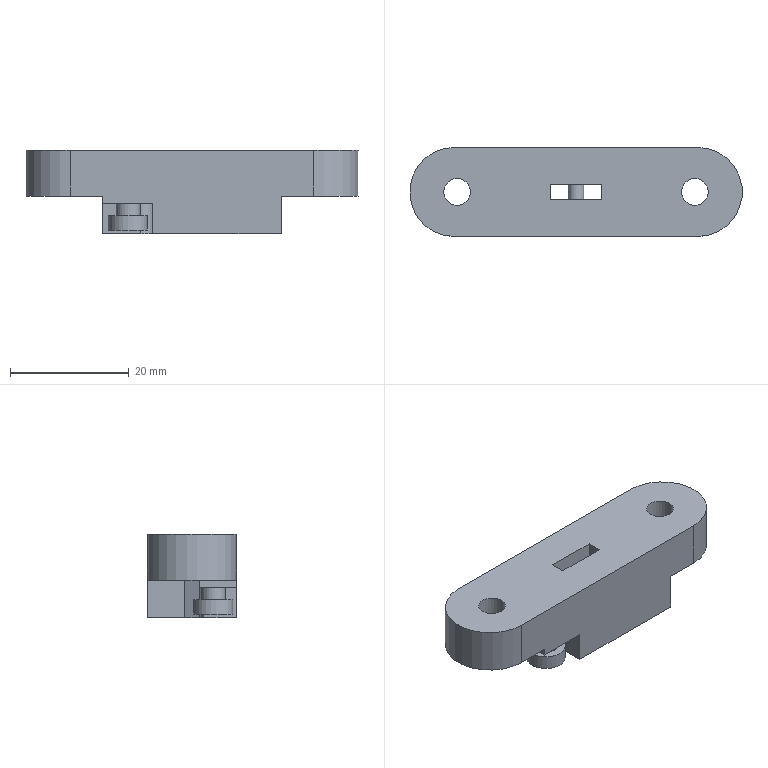Part | NX | 1 solid | 39 faces | box 56 x 15 x 14 mm | volume 7520 mm3 | plane 28 | cylinder 9 | cone 2 | commonest cylinder face diameters 2.7 x2 4 x2 4.5 x2 15 x2 6.6 x1
STEP:
#1=CARTESIAN_POINT('',(2.4,79.3,36.5));
#2=VERTEX_POINT('',#1);
#3=CARTESIAN_POINT('',(4.4,78.54,36.5));
#4=VERTEX_POINT('',#3);
#5=CARTESIAN_POINT('',(4.,80.5,36.5));
#6=DIRECTION('',(0.,0.,-1.));
#7=DIRECTION('',(0.,-1.,0.));
#8=AXIS2_PLACEMENT_3D('',#5,#6,#7);
#9=CIRCLE('',#8,2.);
#10=EDGE_CURVE('',#2,#4,#9,.F.);
#11=ORIENTED_EDGE('',*,*,#10,.T.);
#12=CARTESIAN_POINT('',(4.4,73.,36.5));
#13=VERTEX_POINT('',#12);
#14=CARTESIAN_POINT('',(4.4,79.3,36.5));
#15=DIRECTION('',(0.,-1.,0.));
#16=VECTOR('',#15,1000.);
#17=LINE('',#14,#16);
#18=EDGE_CURVE('',#4,#13,#17,.T.);
#19=ORIENTED_EDGE('',*,*,#18,.T.);
#20=CARTESIAN_POINT('',(-4.,73.,36.5));
#21=VERTEX_POINT('',#20);
#22=CARTESIAN_POINT('',(-4.,73.,36.5));
#23=DIRECTION('',(-1.,0.,0.));
#24=VECTOR('',#23,1000.);
#25=LINE('',#22,#24);
#26=EDGE_CURVE('',#13,#21,#25,.T.);
#27=ORIENTED_EDGE('',*,*,#26,.T.);
#28=CARTESIAN_POINT('',(-4.,79.3,36.5));
#29=VERTEX_POINT('',#28);
#30=CARTESIAN_POINT('',(-4.,79.3,36.5));
#31=DIRECTION('',(0.,1.,0.));
#32=VECTOR('',#31,1000.);
#33=LINE('',#30,#32);
#34=EDGE_CURVE('',#21,#29,#33,.T.);
#35=ORIENTED_EDGE('',*,*,#34,.T.);
#36=CARTESIAN_POINT('',(-4.,79.3,36.5));
#37=DIRECTION('',(1.,0.,0.));
#38=VECTOR('',#37,1000.);
#39=LINE('',#36,#38);
#40=EDGE_CURVE('',#29,#2,#39,.T.);
#41=ORIENTED_EDGE('',*,*,#40,.T.);
#42=EDGE_LOOP('',(#11,#19,#27,#35,#41));
#43=FACE_BOUND('',#42,.T.);
#44=CARTESIAN_POINT('',(0.2,74.9,36.5));
#45=VERTEX_POINT('',#44);
#46=CARTESIAN_POINT('',(0.2,76.9,36.5));
#47=DIRECTION('',(0.,0.,-1.));
#48=DIRECTION('',(0.,-1.,0.));
#49=AXIS2_PLACEMENT_3D('',#46,#47,#48);
#50=CIRCLE('',#49,2.);
#51=EDGE_CURVE('',#45,#45,#50,.T.);
#52=ORIENTED_EDGE('',*,*,#51,.F.);
#53=EDGE_LOOP('',(#52));
#54=FACE_BOUND('',#53,.T.);
#55=CARTESIAN_POINT('',(4.4,79.3,36.5));
#56=DIRECTION('',(0.,0.,-1.));
#57=DIRECTION('',(0.,-1.,0.));
#58=AXIS2_PLACEMENT_3D('',#55,#56,#57);
#59=PLANE('',#58);
#60=ADVANCED_FACE('',(#43,#54),#59,.T.);
#61=ORIENTED_EDGE('',*,*,#34,.F.);
#62=CARTESIAN_POINT('',(-4.,73.,37.7));
#63=VERTEX_POINT('',#62);
#64=CARTESIAN_POINT('',(-4.,73.,31.4));
#65=DIRECTION('',(0.,0.,1.));
#66=VECTOR('',#65,1000.);
#67=LINE('',#64,#66);
#68=EDGE_CURVE('',#21,#63,#67,.T.);
#69=ORIENTED_EDGE('',*,*,#68,.T.);
#70=CARTESIAN_POINT('',(-4.,79.3,37.7));
#71=VERTEX_POINT('',#70);
#72=CARTESIAN_POINT('',(-4.,88.,37.7));
#73=DIRECTION('',(0.,1.,0.));
#74=VECTOR('',#73,1000.);
#75=LINE('',#72,#74);
#76=EDGE_CURVE('',#63,#71,#75,.T.);
#77=ORIENTED_EDGE('',*,*,#76,.T.);
#78=CARTESIAN_POINT('',(-4.,79.3,31.4));
#79=DIRECTION('',(0.,0.,-1.));
#80=VECTOR('',#79,1000.);
#81=LINE('',#78,#80);
#82=EDGE_CURVE('',#71,#29,#81,.T.);
#83=ORIENTED_EDGE('',*,*,#82,.T.);
#84=EDGE_LOOP('',(#61,#69,#77,#83));
#85=FACE_BOUND('',#84,.T.);
#86=CARTESIAN_POINT('',(-4.,88.,31.4));
#87=DIRECTION('',(1.,0.,0.));
#88=DIRECTION('',(0.,0.,1.));
#89=AXIS2_PLACEMENT_3D('',#86,#87,#88);
#90=PLANE('',#89);
#91=ADVANCED_FACE('',(#85),#90,.F.);
#92=CARTESIAN_POINT('',(2.4,79.3,40.7));
#93=VERTEX_POINT('',#92);
#94=CARTESIAN_POINT('',(2.4,79.3,44.4));
#95=DIRECTION('',(0.,0.,-1.));
#96=VECTOR('',#95,1000.);
#97=LINE('',#94,#96);
#98=EDGE_CURVE('',#2,#93,#97,.F.);
#99=ORIENTED_EDGE('',*,*,#98,.F.);
#100=ORIENTED_EDGE('',*,*,#40,.F.);
#101=ORIENTED_EDGE('',*,*,#82,.F.);
#102=CARTESIAN_POINT('',(-4.,79.3,40.7));
#103=VERTEX_POINT('',#102);
#104=CARTESIAN_POINT('',(-4.,79.3,31.4));
#105=DIRECTION('',(0.,0.,-1.));
#106=VECTOR('',#105,1000.);
#107=LINE('',#104,#106);
#108=EDGE_CURVE('',#103,#71,#107,.T.);
#109=ORIENTED_EDGE('',*,*,#108,.F.);
#110=CARTESIAN_POINT('',(-4.,79.3,40.7));
#111=DIRECTION('',(-1.,0.,0.));
#112=VECTOR('',#111,1000.);
#113=LINE('',#110,#112);
#114=EDGE_CURVE('',#93,#103,#113,.T.);
#115=ORIENTED_EDGE('',*,*,#114,.F.);
#116=EDGE_LOOP('',(#99,#100,#101,#109,#115));
#117=FACE_BOUND('',#116,.T.);
#118=CARTESIAN_POINT('',(-4.,79.3,31.4));
#119=DIRECTION('',(0.,1.,0.));
#120=DIRECTION('',(0.,0.,-1.));
#121=AXIS2_PLACEMENT_3D('',#118,#119,#120);
#122=PLANE('',#121);
#123=ADVANCED_FACE('',(#117),#122,.T.);
#124=CARTESIAN_POINT('',(6.7,79.3,40.7));
#125=VERTEX_POINT('',#124);
#126=CARTESIAN_POINT('',(5.6,79.3,40.7));
#127=VERTEX_POINT('',#126);
#128=CARTESIAN_POINT('',(-4.,79.3,40.7));
#129=DIRECTION('',(-1.,0.,0.));
#130=VECTOR('',#129,1000.);
#131=LINE('',#128,#130);
#132=EDGE_CURVE('',#125,#127,#131,.T.);
#133=ORIENTED_EDGE('',*,*,#132,.T.);
#134=CARTESIAN_POINT('',(5.6,81.7,40.7));
#135=VERTEX_POINT('',#134);
#136=CARTESIAN_POINT('',(4.,80.5,40.7));
#137=DIRECTION('',(0.,0.,1.));
#138=DIRECTION('',(-1.,0.,0.));
#139=AXIS2_PLACEMENT_3D('',#136,#137,#138);
#140=CIRCLE('',#139,2.);
#141=EDGE_CURVE('',#127,#135,#140,.T.);
#142=ORIENTED_EDGE('',*,*,#141,.T.);
#143=CARTESIAN_POINT('',(6.7,81.7,40.7));
#144=VERTEX_POINT('',#143);
#145=CARTESIAN_POINT('',(-4.,81.7,40.7));
#146=DIRECTION('',(-1.,0.,0.));
#147=VECTOR('',#146,1000.);
#148=LINE('',#145,#147);
#149=EDGE_CURVE('',#144,#135,#148,.T.);
#150=ORIENTED_EDGE('',*,*,#149,.F.);
#151=CARTESIAN_POINT('',(6.7,81.7,40.7));
#152=DIRECTION('',(0.,-1.,0.));
#153=VECTOR('',#152,1000.);
#154=LINE('',#151,#153);
#155=EDGE_CURVE('',#144,#125,#154,.T.);
#156=ORIENTED_EDGE('',*,*,#155,.T.);
#157=EDGE_LOOP('',(#133,#142,#150,#156));
#158=FACE_BOUND('',#157,.T.);
#159=CARTESIAN_POINT('',(-4.,81.7,40.7));
#160=DIRECTION('',(0.,0.,1.));
#161=DIRECTION('',(-1.,0.,0.));
#162=AXIS2_PLACEMENT_3D('',#159,#160,#161);
#163=PLANE('',#162);
#164=ADVANCED_FACE('',(#158),#163,.F.);
#165=CARTESIAN_POINT('',(11.,81.7,38.85));
#166=VERTEX_POINT('',#165);
#167=CARTESIAN_POINT('',(11.,81.7,40.2));
#168=DIRECTION('',(0.,1.,0.));
#169=DIRECTION('',(0.,0.,-1.));
#170=AXIS2_PLACEMENT_3D('',#167,#168,#169);
#171=CIRCLE('',#170,1.35);
#172=EDGE_CURVE('',#166,#166,#171,.T.);
#173=ORIENTED_EDGE('',*,*,#172,.T.);
#174=EDGE_LOOP('',(#173));
#175=FACE_BOUND('',#174,.T.);
#176=ORIENTED_EDGE('',*,*,#149,.T.);
#177=CARTESIAN_POINT('',(5.6,81.7,31.4));
#178=VERTEX_POINT('',#177);
#179=CARTESIAN_POINT('',(5.6,81.7,44.4));
#180=DIRECTION('',(0.,0.,-1.));
#181=VECTOR('',#180,1000.);
#182=LINE('',#179,#181);
#183=EDGE_CURVE('',#135,#178,#182,.T.);
#184=ORIENTED_EDGE('',*,*,#183,.T.);
#185=CARTESIAN_POINT('',(21.4,81.7,31.4));
#186=VERTEX_POINT('',#185);
#187=CARTESIAN_POINT('',(21.4,81.7,31.4));
#188=DIRECTION('',(1.,0.,0.));
#189=VECTOR('',#188,1000.);
#190=LINE('',#187,#189);
#191=EDGE_CURVE('',#178,#186,#190,.T.);
#192=ORIENTED_EDGE('',*,*,#191,.T.);
#193=CARTESIAN_POINT('',(17.7,81.7,42.5));
#194=VERTEX_POINT('',#193);
#195=CARTESIAN_POINT('',(17.7,81.7,42.5));
#196=DIRECTION('',(-0.3162,0.,0.9487));
#197=VECTOR('',#196,1000.);
#198=LINE('',#195,#197);
#199=EDGE_CURVE('',#186,#194,#198,.T.);
#200=ORIENTED_EDGE('',*,*,#199,.T.);
#201=CARTESIAN_POINT('',(15.3,81.7,42.5));
#202=VERTEX_POINT('',#201);
#203=CARTESIAN_POINT('',(15.3,81.7,42.5));
#204=DIRECTION('',(-1.,0.,0.));
#205=VECTOR('',#204,1000.);
#206=LINE('',#203,#205);
#207=EDGE_CURVE('',#194,#202,#206,.T.);
#208=ORIENTED_EDGE('',*,*,#207,.T.);
#209=CARTESIAN_POINT('',(15.3,81.7,45.4));
#210=VERTEX_POINT('',#209);
#211=CARTESIAN_POINT('',(15.3,81.7,45.4));
#212=DIRECTION('',(0.,0.,1.));
#213=VECTOR('',#212,1000.);
#214=LINE('',#211,#213);
#215=EDGE_CURVE('',#202,#210,#214,.T.);
#216=ORIENTED_EDGE('',*,*,#215,.T.);
#217=CARTESIAN_POINT('',(6.7,81.7,45.4));
#218=VERTEX_POINT('',#217);
#219=CARTESIAN_POINT('',(6.7,81.7,45.4));
#220=DIRECTION('',(-1.,0.,0.));
#221=VECTOR('',#220,1000.);
#222=LINE('',#219,#221);
#223=EDGE_CURVE('',#210,#218,#222,.T.);
#224=ORIENTED_EDGE('',*,*,#223,.T.);
#225=CARTESIAN_POINT('',(6.7,81.7,40.7));
#226=DIRECTION('',(0.,0.,-1.));
#227=VECTOR('',#226,1000.);
#228=LINE('',#225,#227);
#229=EDGE_CURVE('',#218,#144,#228,.T.);
#230=ORIENTED_EDGE('',*,*,#229,.T.);
#231=EDGE_LOOP('',(#176,#184,#192,#200,#208,#216,#224,#230));
#232=FACE_BOUND('',#231,.T.);
#233=CARTESIAN_POINT('',(-4.,81.7,31.4));
#234=DIRECTION('',(0.,1.,0.));
#235=DIRECTION('',(0.,0.,-1.));
#236=AXIS2_PLACEMENT_3D('',#233,#234,#235);
#237=PLANE('',#236);
#238=ADVANCED_FACE('',(#175,#232),#237,.F.);
#239=CARTESIAN_POINT('',(11.,79.3,38.85));
#240=VERTEX_POINT('',#239);
#241=CARTESIAN_POINT('',(11.,79.3,40.2));
#242=DIRECTION('',(0.,1.,0.));
#243=DIRECTION('',(0.,0.,-1.));
#244=AXIS2_PLACEMENT_3D('',#241,#242,#243);
#245=CIRCLE('',#244,1.35);
#246=EDGE_CURVE('',#240,#240,#245,.T.);
#247=ORIENTED_EDGE('',*,*,#246,.F.);
#248=EDGE_LOOP('',(#247));
#249=FACE_BOUND('',#248,.T.);
#250=CARTESIAN_POINT('',(5.6,79.3,31.4));
#251=VERTEX_POINT('',#250);
#252=CARTESIAN_POINT('',(5.6,79.3,44.4));
#253=DIRECTION('',(0.,0.,-1.));
#254=VECTOR('',#253,1000.);
#255=LINE('',#252,#254);
#256=EDGE_CURVE('',#127,#251,#255,.T.);
#257=ORIENTED_EDGE('',*,*,#256,.F.);
#258=ORIENTED_EDGE('',*,*,#132,.F.);
#259=CARTESIAN_POINT('',(6.7,79.3,45.4));
#260=VERTEX_POINT('',#259);
#261=CARTESIAN_POINT('',(6.7,79.3,40.7));
#262=DIRECTION('',(0.,0.,-1.));
#263=VECTOR('',#262,1000.);
#264=LINE('',#261,#263);
#265=EDGE_CURVE('',#260,#125,#264,.T.);
#266=ORIENTED_EDGE('',*,*,#265,.F.);
#267=CARTESIAN_POINT('',(15.3,79.3,45.4));
#268=VERTEX_POINT('',#267);
#269=CARTESIAN_POINT('',(6.7,79.3,45.4));
#270=DIRECTION('',(-1.,0.,0.));
#271=VECTOR('',#270,1000.);
#272=LINE('',#269,#271);
#273=EDGE_CURVE('',#268,#260,#272,.T.);
#274=ORIENTED_EDGE('',*,*,#273,.F.);
#275=CARTESIAN_POINT('',(15.3,79.3,42.5));
#276=VERTEX_POINT('',#275);
#277=CARTESIAN_POINT('',(15.3,79.3,45.4));
#278=DIRECTION('',(0.,0.,1.));
#279=VECTOR('',#278,1000.);
#280=LINE('',#277,#279);
#281=EDGE_CURVE('',#276,#268,#280,.T.);
#282=ORIENTED_EDGE('',*,*,#281,.F.);
#283=CARTESIAN_POINT('',(17.7,79.3,42.5));
#284=VERTEX_POINT('',#283);
#285=CARTESIAN_POINT('',(15.3,79.3,42.5));
#286=DIRECTION('',(-1.,0.,0.));
#287=VECTOR('',#286,1000.);
#288=LINE('',#285,#287);
#289=EDGE_CURVE('',#284,#276,#288,.T.);
#290=ORIENTED_EDGE('',*,*,#289,.F.);
#291=CARTESIAN_POINT('',(21.4,79.3,31.4));
#292=VERTEX_POINT('',#291);
#293=CARTESIAN_POINT('',(17.7,79.3,42.5));
#294=DIRECTION('',(-0.3162,0.,0.9487));
#295=VECTOR('',#294,1000.);
#296=LINE('',#293,#295);
#297=EDGE_CURVE('',#292,#284,#296,.T.);
#298=ORIENTED_EDGE('',*,*,#297,.F.);
#299=CARTESIAN_POINT('',(21.4,79.3,31.4));
#300=DIRECTION('',(1.,0.,0.));
#301=VECTOR('',#300,1000.);
#302=LINE('',#299,#301);
#303=EDGE_CURVE('',#251,#292,#302,.T.);
#304=ORIENTED_EDGE('',*,*,#303,.F.);
#305=EDGE_LOOP('',(#257,#258,#266,#274,#282,#290,#298,#304));
#306=FACE_BOUND('',#305,.T.);
#307=CARTESIAN_POINT('',(-4.,79.3,31.4));
#308=DIRECTION('',(0.,1.,0.));
#309=DIRECTION('',(0.,0.,-1.));
#310=AXIS2_PLACEMENT_3D('',#307,#308,#309);
#311=PLANE('',#310);
#312=ADVANCED_FACE('',(#249,#306),#311,.T.);
#313=CARTESIAN_POINT('',(-9.,85.,37.7));
#314=VERTEX_POINT('',#313);
#315=CARTESIAN_POINT('',(-9.,80.5,37.7));
#316=DIRECTION('',(0.,0.,1.));
#317=DIRECTION('',(0.,1.,0.));
#318=AXIS2_PLACEMENT_3D('',#315,#316,#317);
#319=CIRCLE('',#318,4.5);
#320=EDGE_CURVE('',#314,#314,#319,.T.);
#321=ORIENTED_EDGE('',*,*,#320,.T.);
#322=EDGE_LOOP('',(#321));
#323=FACE_BOUND('',#322,.T.);
#324=ORIENTED_EDGE('',*,*,#76,.F.);
#325=CARTESIAN_POINT('',(-9.5,73.,37.7));
#326=VERTEX_POINT('',#325);
#327=CARTESIAN_POINT('',(-9.5,73.,37.7));
#328=DIRECTION('',(-1.,0.,0.));
#329=VECTOR('',#328,1000.);
#330=LINE('',#327,#329);
#331=EDGE_CURVE('',#63,#326,#330,.T.);
#332=ORIENTED_EDGE('',*,*,#331,.T.);
#333=CARTESIAN_POINT('',(-9.5,88.,37.7));
#334=VERTEX_POINT('',#333);
#335=CARTESIAN_POINT('',(-9.5,80.5,37.7));
#336=DIRECTION('',(0.,0.,-1.));
#337=DIRECTION('',(0.,1.,0.));
#338=AXIS2_PLACEMENT_3D('',#335,#336,#337);
#339=CIRCLE('',#338,7.5);
#340=EDGE_CURVE('',#326,#334,#339,.T.);
#341=ORIENTED_EDGE('',*,*,#340,.T.);
#342=CARTESIAN_POINT('',(-4.,88.,37.7));
#343=VERTEX_POINT('',#342);
#344=CARTESIAN_POINT('',(-9.5,88.,37.7));
#345=DIRECTION('',(1.,0.,0.));
#346=VECTOR('',#345,1000.);
#347=LINE('',#344,#346);
#348=EDGE_CURVE('',#334,#343,#347,.T.);
#349=ORIENTED_EDGE('',*,*,#348,.T.);
#350=CARTESIAN_POINT('',(-4.,81.7,37.7));
#351=VERTEX_POINT('',#350);
#352=CARTESIAN_POINT('',(-4.,88.,37.7));
#353=DIRECTION('',(0.,1.,0.));
#354=VECTOR('',#353,1000.);
#355=LINE('',#352,#354);
#356=EDGE_CURVE('',#351,#343,#355,.T.);
#357=ORIENTED_EDGE('',*,*,#356,.F.);
#358=CARTESIAN_POINT('',(-4.,80.5,37.7));
#359=DIRECTION('',(0.,-1.,0.));
#360=VECTOR('',#359,1000.);
#361=LINE('',#358,#360);
#362=EDGE_CURVE('',#351,#71,#361,.T.);
#363=ORIENTED_EDGE('',*,*,#362,.T.);
#364=EDGE_LOOP('',(#324,#332,#341,#349,#357,#363));
#365=FACE_BOUND('',#364,.T.);
#366=CARTESIAN_POINT('',(-9.5,80.5,37.7));
#367=DIRECTION('',(0.,0.,1.));
#368=DIRECTION('',(0.,1.,0.));
#369=AXIS2_PLACEMENT_3D('',#366,#367,#368);
#370=PLANE('',#369);
#371=ADVANCED_FACE('',(#323,#365),#370,.F.);
#372=CARTESIAN_POINT('',(31.,85.,37.7));
#373=VERTEX_POINT('',#372);
#374=CARTESIAN_POINT('',(31.,80.5,37.7));
#375=DIRECTION('',(0.,0.,1.));
#376=DIRECTION('',(0.,1.,0.));
#377=AXIS2_PLACEMENT_3D('',#374,#375,#376);
#378=CIRCLE('',#377,4.5);
#379=EDGE_CURVE('',#373,#373,#378,.T.);
#380=ORIENTED_EDGE('',*,*,#379,.T.);
#381=EDGE_LOOP('',(#380));
#382=FACE_BOUND('',#381,.T.);
#383=CARTESIAN_POINT('',(26.,88.,37.7));
#384=VERTEX_POINT('',#383);
#385=CARTESIAN_POINT('',(26.,73.,37.7));
#386=VERTEX_POINT('',#385);
#387=CARTESIAN_POINT('',(26.,88.,37.7));
#388=DIRECTION('',(0.,-1.,0.));
#389=VECTOR('',#388,1000.);
#390=LINE('',#387,#389);
#391=EDGE_CURVE('',#384,#386,#390,.T.);
#392=ORIENTED_EDGE('',*,*,#391,.F.);
#393=CARTESIAN_POINT('',(31.5,88.,37.7));
#394=VERTEX_POINT('',#393);
#395=CARTESIAN_POINT('',(-9.5,88.,37.7));
#396=DIRECTION('',(1.,0.,0.));
#397=VECTOR('',#396,1000.);
#398=LINE('',#395,#397);
#399=EDGE_CURVE('',#384,#394,#398,.T.);
#400=ORIENTED_EDGE('',*,*,#399,.T.);
#401=CARTESIAN_POINT('',(31.5,73.,37.7));
#402=VERTEX_POINT('',#401);
#403=CARTESIAN_POINT('',(31.5,80.5,37.7));
#404=DIRECTION('',(0.,0.,-1.));
#405=DIRECTION('',(0.,1.,0.));
#406=AXIS2_PLACEMENT_3D('',#403,#404,#405);
#407=CIRCLE('',#406,7.5);
#408=EDGE_CURVE('',#394,#402,#407,.T.);
#409=ORIENTED_EDGE('',*,*,#408,.T.);
#410=CARTESIAN_POINT('',(-9.5,73.,37.7));
#411=DIRECTION('',(-1.,0.,0.));
#412=VECTOR('',#411,1000.);
#413=LINE('',#410,#412);
#414=EDGE_CURVE('',#402,#386,#413,.T.);
#415=ORIENTED_EDGE('',*,*,#414,.T.);
#416=EDGE_LOOP('',(#392,#400,#409,#415));
#417=FACE_BOUND('',#416,.T.);
#418=CARTESIAN_POINT('',(-9.5,80.5,37.7));
#419=DIRECTION('',(0.,0.,1.));
#420=DIRECTION('',(0.,1.,0.));
#421=AXIS2_PLACEMENT_3D('',#418,#419,#420);
#422=PLANE('',#421);
#423=ADVANCED_FACE('',(#382,#417),#422,.F.);
#424=CARTESIAN_POINT('',(-9.5,73.,45.4));
#425=VERTEX_POINT('',#424);
#426=CARTESIAN_POINT('',(-9.5,88.,45.4));
#427=VERTEX_POINT('',#426);
#428=CARTESIAN_POINT('',(-9.5,80.5,45.4));
#429=DIRECTION('',(0.,0.,-1.));
#430=DIRECTION('',(0.,1.,0.));
#431=AXIS2_PLACEMENT_3D('',#428,#429,#430);
#432=CIRCLE('',#431,7.5);
#433=EDGE_CURVE('',#425,#427,#432,.T.);
#434=ORIENTED_EDGE('',*,*,#433,.T.);
#435=CARTESIAN_POINT('',(-9.5,88.,37.7));
#436=DIRECTION('',(0.,0.,1.));
#437=VECTOR('',#436,1000.);
#438=LINE('',#435,#437);
#439=EDGE_CURVE('',#334,#427,#438,.T.);
#440=ORIENTED_EDGE('',*,*,#439,.F.);
#441=ORIENTED_EDGE('',*,*,#340,.F.);
#442=CARTESIAN_POINT('',(-9.5,73.,37.7));
#443=DIRECTION('',(0.,0.,1.));
#444=VECTOR('',#443,1000.);
#445=LINE('',#442,#444);
#446=EDGE_CURVE('',#326,#425,#445,.T.);
#447=ORIENTED_EDGE('',*,*,#446,.T.);
#448=EDGE_LOOP('',(#434,#440,#441,#447));
#449=FACE_BOUND('',#448,.T.);
#450=CARTESIAN_POINT('',(-9.5,80.5,37.7));
#451=DIRECTION('',(0.,0.,1.));
#452=DIRECTION('',(0.,1.,0.));
#453=AXIS2_PLACEMENT_3D('',#450,#451,#452);
#454=CYLINDRICAL_SURFACE('',#453,7.5);
#455=ADVANCED_FACE('',(#449),#454,.T.);
#456=CARTESIAN_POINT('',(11.,88.,38.85));
#457=VERTEX_POINT('',#456);
#458=CARTESIAN_POINT('',(11.,88.,40.2));
#459=DIRECTION('',(0.,1.,0.));
#460=DIRECTION('',(0.,0.,-1.));
#461=AXIS2_PLACEMENT_3D('',#458,#459,#460);
#462=CIRCLE('',#461,1.35);
#463=EDGE_CURVE('',#457,#457,#462,.T.);
#464=ORIENTED_EDGE('',*,*,#463,.F.);
#465=EDGE_LOOP('',(#464));
#466=FACE_BOUND('',#465,.T.);
#467=CARTESIAN_POINT('',(31.5,88.,45.4));
#468=VERTEX_POINT('',#467);
#469=CARTESIAN_POINT('',(-9.5,88.,45.4));
#470=DIRECTION('',(1.,0.,0.));
#471=VECTOR('',#470,1000.);
#472=LINE('',#469,#471);
#473=EDGE_CURVE('',#427,#468,#472,.T.);
#474=ORIENTED_EDGE('',*,*,#473,.T.);
#475=CARTESIAN_POINT('',(31.5,88.,37.7));
#476=DIRECTION('',(0.,0.,1.));
#477=VECTOR('',#476,1000.);
#478=LINE('',#475,#477);
#479=EDGE_CURVE('',#394,#468,#478,.T.);
#480=ORIENTED_EDGE('',*,*,#479,.F.);
#481=ORIENTED_EDGE('',*,*,#399,.F.);
#482=CARTESIAN_POINT('',(26.,88.,31.4));
#483=VERTEX_POINT('',#482);
#484=CARTESIAN_POINT('',(26.,88.,31.4));
#485=DIRECTION('',(0.,0.,1.));
#486=VECTOR('',#485,1000.);
#487=LINE('',#484,#486);
#488=EDGE_CURVE('',#483,#384,#487,.T.);
#489=ORIENTED_EDGE('',*,*,#488,.F.);
#490=CARTESIAN_POINT('',(-4.,88.,31.4));
#491=VERTEX_POINT('',#490);
#492=CARTESIAN_POINT('',(-4.,88.,31.4));
#493=DIRECTION('',(1.,0.,0.));
#494=VECTOR('',#493,1000.);
#495=LINE('',#492,#494);
#496=EDGE_CURVE('',#491,#483,#495,.T.);
#497=ORIENTED_EDGE('',*,*,#496,.F.);
#498=CARTESIAN_POINT('',(-4.,88.,31.4));
#499=DIRECTION('',(0.,0.,1.));
#500=VECTOR('',#499,1000.);
#501=LINE('',#498,#500);
#502=EDGE_CURVE('',#491,#343,#501,.T.);
#503=ORIENTED_EDGE('',*,*,#502,.T.);
#504=ORIENTED_EDGE('',*,*,#348,.F.);
#505=ORIENTED_EDGE('',*,*,#439,.T.);
#506=EDGE_LOOP('',(#474,#480,#481,#489,#497,#503,#504,#505));
#507=FACE_BOUND('',#506,.T.);
#508=CARTESIAN_POINT('',(-9.5,88.,37.7));
#509=DIRECTION('',(0.,-1.,0.));
#510=DIRECTION('',(0.,0.,1.));
#511=AXIS2_PLACEMENT_3D('',#508,#509,#510);
#512=PLANE('',#511);
#513=ADVANCED_FACE('',(#466,#507),#512,.F.);
#514=CARTESIAN_POINT('',(31.5,73.,45.4));
#515=VERTEX_POINT('',#514);
#516=CARTESIAN_POINT('',(31.5,80.5,45.4));
#517=DIRECTION('',(0.,0.,-1.));
#518=DIRECTION('',(0.,1.,0.));
#519=AXIS2_PLACEMENT_3D('',#516,#517,#518);
#520=CIRCLE('',#519,7.5);
#521=EDGE_CURVE('',#468,#515,#520,.T.);
#522=ORIENTED_EDGE('',*,*,#521,.T.);
#523=CARTESIAN_POINT('',(31.5,73.,37.7));
#524=DIRECTION('',(0.,0.,1.));
#525=VECTOR('',#524,1000.);
#526=LINE('',#523,#525);
#527=EDGE_CURVE('',#402,#515,#526,.T.);
#528=ORIENTED_EDGE('',*,*,#527,.F.);
#529=ORIENTED_EDGE('',*,*,#408,.F.);
#530=ORIENTED_EDGE('',*,*,#479,.T.);
#531=EDGE_LOOP('',(#522,#528,#529,#530));
#532=FACE_BOUND('',#531,.T.);
#533=CARTESIAN_POINT('',(31.5,80.5,37.7));
#534=DIRECTION('',(0.,0.,1.));
#535=DIRECTION('',(0.,1.,0.));
#536=AXIS2_PLACEMENT_3D('',#533,#534,#535);
#537=CYLINDRICAL_SURFACE('',#536,7.5);
#538=ADVANCED_FACE('',(#532),#537,.T.);
#539=ORIENTED_EDGE('',*,*,#26,.F.);
#540=CARTESIAN_POINT('',(4.4,73.,31.4));
#541=VERTEX_POINT('',#540);
#542=CARTESIAN_POINT('',(4.4,73.,36.5));
#543=DIRECTION('',(0.,0.,-1.));
#544=VECTOR('',#543,1000.);
#545=LINE('',#542,#544);
#546=EDGE_CURVE('',#13,#541,#545,.T.);
#547=ORIENTED_EDGE('',*,*,#546,.T.);
#548=CARTESIAN_POINT('',(26.,73.,31.4));
#549=VERTEX_POINT('',#548);
#550=CARTESIAN_POINT('',(-4.,73.,31.4));
#551=DIRECTION('',(-1.,0.,0.));
#552=VECTOR('',#551,1000.);
#553=LINE('',#550,#552);
#554=EDGE_CURVE('',#549,#541,#553,.T.);
#555=ORIENTED_EDGE('',*,*,#554,.F.);
#556=CARTESIAN_POINT('',(26.,73.,31.4));
#557=DIRECTION('',(0.,0.,1.));
#558=VECTOR('',#557,1000.);
#559=LINE('',#556,#558);
#560=EDGE_CURVE('',#549,#386,#559,.T.);
#561=ORIENTED_EDGE('',*,*,#560,.T.);
#562=ORIENTED_EDGE('',*,*,#414,.F.);
#563=ORIENTED_EDGE('',*,*,#527,.T.);
#564=CARTESIAN_POINT('',(-9.5,73.,45.4));
#565=DIRECTION('',(-1.,0.,0.));
#566=VECTOR('',#565,1000.);
#567=LINE('',#564,#566);
#568=EDGE_CURVE('',#515,#425,#567,.T.);
#569=ORIENTED_EDGE('',*,*,#568,.T.);
#570=ORIENTED_EDGE('',*,*,#446,.F.);
#571=ORIENTED_EDGE('',*,*,#331,.F.);
#572=ORIENTED_EDGE('',*,*,#68,.F.);
#573=EDGE_LOOP('',(#539,#547,#555,#561,#562,#563,#569,#570,#571,#572));
#574=FACE_BOUND('',#573,.T.);
#575=CARTESIAN_POINT('',(-9.5,73.,37.7));
#576=DIRECTION('',(0.,1.,0.));
#577=DIRECTION('',(0.,0.,-1.));
#578=AXIS2_PLACEMENT_3D('',#575,#576,#577);
#579=PLANE('',#578);
#580=ADVANCED_FACE('',(#574),#579,.F.);
#581=ORIENTED_EDGE('',*,*,#223,.F.);
#582=CARTESIAN_POINT('',(15.3,81.7,45.4));
#583=DIRECTION('',(0.,-1.,0.));
#584=VECTOR('',#583,1000.);
#585=LINE('',#582,#584);
#586=EDGE_CURVE('',#210,#268,#585,.T.);
#587=ORIENTED_EDGE('',*,*,#586,.T.);
#588=ORIENTED_EDGE('',*,*,#273,.T.);
#589=CARTESIAN_POINT('',(6.7,81.7,45.4));
#590=DIRECTION('',(0.,-1.,0.));
#591=VECTOR('',#590,1000.);
#592=LINE('',#589,#591);
#593=EDGE_CURVE('',#218,#260,#592,.T.);
#594=ORIENTED_EDGE('',*,*,#593,.F.);
#595=EDGE_LOOP('',(#581,#587,#588,#594));
#596=FACE_BOUND('',#595,.T.);
#597=CARTESIAN_POINT('',(31.,82.75,45.4));
#598=VERTEX_POINT('',#597);
#599=CARTESIAN_POINT('',(31.,80.5,45.4));
#600=DIRECTION('',(0.,0.,1.));
#601=DIRECTION('',(0.,1.,0.));
#602=AXIS2_PLACEMENT_3D('',#599,#600,#601);
#603=CIRCLE('',#602,2.25);
#604=EDGE_CURVE('',#598,#598,#603,.T.);
#605=ORIENTED_EDGE('',*,*,#604,.F.);
#606=EDGE_LOOP('',(#605));
#607=FACE_BOUND('',#606,.T.);
#608=CARTESIAN_POINT('',(-9.,82.75,45.4));
#609=VERTEX_POINT('',#608);
#610=CARTESIAN_POINT('',(-9.,80.5,45.4));
#611=DIRECTION('',(0.,0.,1.));
#612=DIRECTION('',(0.,1.,0.));
#613=AXIS2_PLACEMENT_3D('',#610,#611,#612);
#614=CIRCLE('',#613,2.25);
#615=EDGE_CURVE('',#609,#609,#614,.T.);
#616=ORIENTED_EDGE('',*,*,#615,.F.);
#617=EDGE_LOOP('',(#616));
#618=FACE_BOUND('',#617,.T.);
#619=ORIENTED_EDGE('',*,*,#433,.F.);
#620=ORIENTED_EDGE('',*,*,#568,.F.);
#621=ORIENTED_EDGE('',*,*,#521,.F.);
#622=ORIENTED_EDGE('',*,*,#473,.F.);
#623=EDGE_LOOP('',(#619,#620,#621,#622));
#624=FACE_BOUND('',#623,.T.);
#625=CARTESIAN_POINT('',(-9.5,80.5,45.4));
#626=DIRECTION('',(0.,0.,1.));
#627=DIRECTION('',(0.,1.,0.));
#628=AXIS2_PLACEMENT_3D('',#625,#626,#627);
#629=PLANE('',#628);
#630=ADVANCED_FACE('',(#596,#607,#618,#624),#629,.T.);
#631=ORIENTED_EDGE('',*,*,#320,.F.);
#632=EDGE_LOOP('',(#631));
#633=FACE_BOUND('',#632,.T.);
#634=CARTESIAN_POINT('',(-9.,84.5,41.4));
#635=VERTEX_POINT('',#634);
#636=CARTESIAN_POINT('',(-9.,80.5,41.4));
#637=DIRECTION('',(0.,0.,1.));
#638=DIRECTION('',(0.,1.,0.));
#639=AXIS2_PLACEMENT_3D('',#636,#637,#638);
#640=CIRCLE('',#639,4.);
#641=EDGE_CURVE('',#635,#635,#640,.T.);
#642=ORIENTED_EDGE('',*,*,#641,.T.);
#643=EDGE_LOOP('',(#642));
#644=FACE_BOUND('',#643,.T.);
#645=CARTESIAN_POINT('',(-9.,80.5,41.4));
#646=DIRECTION('',(0.,0.,-1.));
#647=DIRECTION('',(0.,-1.,0.));
#648=AXIS2_PLACEMENT_3D('',#645,#646,#647);
#649=CONICAL_SURFACE('',#648,4.,0.1343);
#650=ADVANCED_FACE('',(#633,#644),#649,.F.);
#651=ORIENTED_EDGE('',*,*,#641,.F.);
#652=EDGE_LOOP('',(#651));
#653=FACE_BOUND('',#652,.T.);
#654=CARTESIAN_POINT('',(-9.,82.75,41.4));
#655=VERTEX_POINT('',#654);
#656=CARTESIAN_POINT('',(-9.,80.5,41.4));
#657=DIRECTION('',(0.,0.,1.));
#658=DIRECTION('',(0.,1.,0.));
#659=AXIS2_PLACEMENT_3D('',#656,#657,#658);
#660=CIRCLE('',#659,2.25);
#661=EDGE_CURVE('',#655,#655,#660,.T.);
#662=ORIENTED_EDGE('',*,*,#661,.T.);
#663=EDGE_LOOP('',(#662));
#664=FACE_BOUND('',#663,.T.);
#665=CARTESIAN_POINT('',(-11.25,80.5,41.4));
#666=DIRECTION('',(0.,0.,1.));
#667=DIRECTION('',(0.,1.,0.));
#668=AXIS2_PLACEMENT_3D('',#665,#666,#667);
#669=PLANE('',#668);
#670=ADVANCED_FACE('',(#653,#664),#669,.F.);
#671=ORIENTED_EDGE('',*,*,#661,.F.);
#672=EDGE_LOOP('',(#671));
#673=FACE_BOUND('',#672,.T.);
#674=ORIENTED_EDGE('',*,*,#615,.T.);
#675=EDGE_LOOP('',(#674));
#676=FACE_BOUND('',#675,.T.);
#677=CARTESIAN_POINT('',(-9.,80.5,51.721));
#678=DIRECTION('',(0.,0.,1.));
#679=DIRECTION('',(0.,1.,0.));
#680=AXIS2_PLACEMENT_3D('',#677,#678,#679);
#681=CYLINDRICAL_SURFACE('',#680,2.25);
#682=ADVANCED_FACE('',(#673,#676),#681,.F.);
#683=ORIENTED_EDGE('',*,*,#379,.F.);
#684=EDGE_LOOP('',(#683));
#685=FACE_BOUND('',#684,.T.);
#686=CARTESIAN_POINT('',(31.,84.5,41.4));
#687=VERTEX_POINT('',#686);
#688=CARTESIAN_POINT('',(31.,80.5,41.4));
#689=DIRECTION('',(0.,0.,1.));
#690=DIRECTION('',(0.,1.,0.));
#691=AXIS2_PLACEMENT_3D('',#688,#689,#690);
#692=CIRCLE('',#691,4.);
#693=EDGE_CURVE('',#687,#687,#692,.T.);
#694=ORIENTED_EDGE('',*,*,#693,.T.);
#695=EDGE_LOOP('',(#694));
#696=FACE_BOUND('',#695,.T.);
#697=CARTESIAN_POINT('',(31.,80.5,41.4));
#698=DIRECTION('',(0.,0.,-1.));
#699=DIRECTION('',(0.,-1.,0.));
#700=AXIS2_PLACEMENT_3D('',#697,#698,#699);
#701=CONICAL_SURFACE('',#700,4.,0.1343);
#702=ADVANCED_FACE('',(#685,#696),#701,.F.);
#703=ORIENTED_EDGE('',*,*,#693,.F.);
#704=EDGE_LOOP('',(#703));
#705=FACE_BOUND('',#704,.T.);
#706=CARTESIAN_POINT('',(31.,82.75,41.4));
#707=VERTEX_POINT('',#706);
#708=CARTESIAN_POINT('',(31.,80.5,41.4));
#709=DIRECTION('',(0.,0.,1.));
#710=DIRECTION('',(0.,1.,0.));
#711=AXIS2_PLACEMENT_3D('',#708,#709,#710);
#712=CIRCLE('',#711,2.25);
#713=EDGE_CURVE('',#707,#707,#712,.T.);
#714=ORIENTED_EDGE('',*,*,#713,.T.);
#715=EDGE_LOOP('',(#714));
#716=FACE_BOUND('',#715,.T.);
#717=CARTESIAN_POINT('',(28.75,80.5,41.4));
#718=DIRECTION('',(0.,0.,1.));
#719=DIRECTION('',(0.,1.,0.));
#720=AXIS2_PLACEMENT_3D('',#717,#718,#719);
#721=PLANE('',#720);
#722=ADVANCED_FACE('',(#705,#716),#721,.F.);
#723=ORIENTED_EDGE('',*,*,#713,.F.);
#724=EDGE_LOOP('',(#723));
#725=FACE_BOUND('',#724,.T.);
#726=ORIENTED_EDGE('',*,*,#604,.T.);
#727=EDGE_LOOP('',(#726));
#728=FACE_BOUND('',#727,.T.);
#729=CARTESIAN_POINT('',(31.,80.5,51.721));
#730=DIRECTION('',(0.,0.,1.));
#731=DIRECTION('',(0.,1.,0.));
#732=AXIS2_PLACEMENT_3D('',#729,#730,#731);
#733=CYLINDRICAL_SURFACE('',#732,2.25);
#734=ADVANCED_FACE('',(#725,#728),#733,.F.);
#735=ORIENTED_EDGE('',*,*,#391,.T.);
#736=ORIENTED_EDGE('',*,*,#560,.F.);
#737=CARTESIAN_POINT('',(26.,88.,31.4));
#738=DIRECTION('',(0.,-1.,0.));
#739=VECTOR('',#738,1000.);
#740=LINE('',#737,#739);
#741=EDGE_CURVE('',#483,#549,#740,.T.);
#742=ORIENTED_EDGE('',*,*,#741,.F.);
#743=ORIENTED_EDGE('',*,*,#488,.T.);
#744=EDGE_LOOP('',(#735,#736,#742,#743));
#745=FACE_BOUND('',#744,.T.);
#746=CARTESIAN_POINT('',(26.,88.,31.4));
#747=DIRECTION('',(-1.,0.,0.));
#748=DIRECTION('',(0.,0.,-1.));
#749=AXIS2_PLACEMENT_3D('',#746,#747,#748);
#750=PLANE('',#749);
#751=ADVANCED_FACE('',(#745),#750,.F.);
#752=CARTESIAN_POINT('',(-4.,81.7,31.4));
#753=VERTEX_POINT('',#752);
#754=CARTESIAN_POINT('',(-4.,88.,31.4));
#755=DIRECTION('',(0.,1.,0.));
#756=VECTOR('',#755,1000.);
#757=LINE('',#754,#756);
#758=EDGE_CURVE('',#753,#491,#757,.T.);
#759=ORIENTED_EDGE('',*,*,#758,.F.);
#760=CARTESIAN_POINT('',(-4.,81.7,31.4));
#761=DIRECTION('',(0.,0.,-1.));
#762=VECTOR('',#761,1000.);
#763=LINE('',#760,#762);
#764=EDGE_CURVE('',#351,#753,#763,.T.);
#765=ORIENTED_EDGE('',*,*,#764,.F.);
#766=ORIENTED_EDGE('',*,*,#356,.T.);
#767=ORIENTED_EDGE('',*,*,#502,.F.);
#768=EDGE_LOOP('',(#759,#765,#766,#767));
#769=FACE_BOUND('',#768,.T.);
#770=CARTESIAN_POINT('',(-4.,88.,31.4));
#771=DIRECTION('',(1.,0.,0.));
#772=DIRECTION('',(0.,0.,1.));
#773=AXIS2_PLACEMENT_3D('',#770,#771,#772);
#774=PLANE('',#773);
#775=ADVANCED_FACE('',(#769),#774,.F.);
#776=CARTESIAN_POINT('',(4.4,78.54,31.4));
#777=VERTEX_POINT('',#776);
#778=CARTESIAN_POINT('',(4.4,79.3,31.4));
#779=DIRECTION('',(0.,-1.,0.));
#780=VECTOR('',#779,1000.);
#781=LINE('',#778,#780);
#782=EDGE_CURVE('',#777,#541,#781,.T.);
#783=ORIENTED_EDGE('',*,*,#782,.F.);
#784=CARTESIAN_POINT('',(4.,80.5,31.4));
#785=DIRECTION('',(0.,0.,-1.));
#786=DIRECTION('',(0.,-1.,0.));
#787=AXIS2_PLACEMENT_3D('',#784,#785,#786);
#788=CIRCLE('',#787,2.);
#789=EDGE_CURVE('',#251,#777,#788,.T.);
#790=ORIENTED_EDGE('',*,*,#789,.F.);
#791=ORIENTED_EDGE('',*,*,#303,.T.);
#792=CARTESIAN_POINT('',(21.4,81.7,31.4));
#793=DIRECTION('',(0.,-1.,0.));
#794=VECTOR('',#793,1000.);
#795=LINE('',#792,#794);
#796=EDGE_CURVE('',#186,#292,#795,.T.);
#797=ORIENTED_EDGE('',*,*,#796,.F.);
#798=ORIENTED_EDGE('',*,*,#191,.F.);
#799=CARTESIAN_POINT('',(2.4,81.7,31.4));
#800=VERTEX_POINT('',#799);
#801=CARTESIAN_POINT('',(4.,80.5,31.4));
#802=DIRECTION('',(0.,0.,-1.));
#803=DIRECTION('',(0.,-1.,0.));
#804=AXIS2_PLACEMENT_3D('',#801,#802,#803);
#805=CIRCLE('',#804,2.);
#806=EDGE_CURVE('',#800,#178,#805,.T.);
#807=ORIENTED_EDGE('',*,*,#806,.F.);
#808=CARTESIAN_POINT('',(21.4,81.7,31.4));
#809=DIRECTION('',(1.,0.,0.));
#810=VECTOR('',#809,1000.);
#811=LINE('',#808,#810);
#812=EDGE_CURVE('',#753,#800,#811,.T.);
#813=ORIENTED_EDGE('',*,*,#812,.F.);
#814=ORIENTED_EDGE('',*,*,#758,.T.);
#815=ORIENTED_EDGE('',*,*,#496,.T.);
#816=ORIENTED_EDGE('',*,*,#741,.T.);
#817=ORIENTED_EDGE('',*,*,#554,.T.);
#818=EDGE_LOOP('',(#783,#790,#791,#797,#798,#807,#813,#814,#815,#816,#817));
#819=FACE_BOUND('',#818,.T.);
#820=CARTESIAN_POINT('',(26.,88.,31.4));
#821=DIRECTION('',(0.,0.,-1.));
#822=DIRECTION('',(0.,-1.,0.));
#823=AXIS2_PLACEMENT_3D('',#820,#821,#822);
#824=PLANE('',#823);
#825=ADVANCED_FACE('',(#819),#824,.T.);
#826=CARTESIAN_POINT('',(-4.,81.7,40.7));
#827=VERTEX_POINT('',#826);
#828=CARTESIAN_POINT('',(-4.,81.7,31.4));
#829=DIRECTION('',(0.,0.,-1.));
#830=VECTOR('',#829,1000.);
#831=LINE('',#828,#830);
#832=EDGE_CURVE('',#827,#351,#831,.T.);
#833=ORIENTED_EDGE('',*,*,#832,.F.);
#834=CARTESIAN_POINT('',(-4.,81.7,40.7));
#835=DIRECTION('',(0.,-1.,0.));
#836=VECTOR('',#835,1000.);
#837=LINE('',#834,#836);
#838=EDGE_CURVE('',#827,#103,#837,.T.);
#839=ORIENTED_EDGE('',*,*,#838,.T.);
#840=ORIENTED_EDGE('',*,*,#108,.T.);
#841=ORIENTED_EDGE('',*,*,#362,.F.);
#842=EDGE_LOOP('',(#833,#839,#840,#841));
#843=FACE_BOUND('',#842,.T.);
#844=CARTESIAN_POINT('',(-4.,81.7,31.4));
#845=DIRECTION('',(-1.,0.,0.));
#846=DIRECTION('',(0.,0.,-1.));
#847=AXIS2_PLACEMENT_3D('',#844,#845,#846);
#848=PLANE('',#847);
#849=ADVANCED_FACE('',(#843),#848,.F.);
#850=CARTESIAN_POINT('',(2.4,81.7,40.7));
#851=VERTEX_POINT('',#850);
#852=CARTESIAN_POINT('',(-4.,81.7,40.7));
#853=DIRECTION('',(-1.,0.,0.));
#854=VECTOR('',#853,1000.);
#855=LINE('',#852,#854);
#856=EDGE_CURVE('',#851,#827,#855,.T.);
#857=ORIENTED_EDGE('',*,*,#856,.F.);
#858=CARTESIAN_POINT('',(4.,80.5,40.7));
#859=DIRECTION('',(0.,0.,1.));
#860=DIRECTION('',(-1.,0.,0.));
#861=AXIS2_PLACEMENT_3D('',#858,#859,#860);
#862=CIRCLE('',#861,2.);
#863=EDGE_CURVE('',#851,#93,#862,.T.);
#864=ORIENTED_EDGE('',*,*,#863,.T.);
#865=ORIENTED_EDGE('',*,*,#114,.T.);
#866=ORIENTED_EDGE('',*,*,#838,.F.);
#867=EDGE_LOOP('',(#857,#864,#865,#866));
#868=FACE_BOUND('',#867,.T.);
#869=CARTESIAN_POINT('',(-4.,81.7,40.7));
#870=DIRECTION('',(0.,0.,1.));
#871=DIRECTION('',(-1.,0.,0.));
#872=AXIS2_PLACEMENT_3D('',#869,#870,#871);
#873=PLANE('',#872);
#874=ADVANCED_FACE('',(#868),#873,.F.);
#875=ORIENTED_EDGE('',*,*,#265,.T.);
#876=ORIENTED_EDGE('',*,*,#155,.F.);
#877=ORIENTED_EDGE('',*,*,#229,.F.);
#878=ORIENTED_EDGE('',*,*,#593,.T.);
#879=EDGE_LOOP('',(#875,#876,#877,#878));
#880=FACE_BOUND('',#879,.T.);
#881=CARTESIAN_POINT('',(6.7,81.7,40.7));
#882=DIRECTION('',(-1.,0.,0.));
#883=DIRECTION('',(0.,0.,-1.));
#884=AXIS2_PLACEMENT_3D('',#881,#882,#883);
#885=PLANE('',#884);
#886=ADVANCED_FACE('',(#880),#885,.F.);
#887=ORIENTED_EDGE('',*,*,#281,.T.);
#888=ORIENTED_EDGE('',*,*,#586,.F.);
#889=ORIENTED_EDGE('',*,*,#215,.F.);
#890=CARTESIAN_POINT('',(15.3,81.7,42.5));
#891=DIRECTION('',(0.,-1.,0.));
#892=VECTOR('',#891,1000.);
#893=LINE('',#890,#892);
#894=EDGE_CURVE('',#202,#276,#893,.T.);
#895=ORIENTED_EDGE('',*,*,#894,.T.);
#896=EDGE_LOOP('',(#887,#888,#889,#895));
#897=FACE_BOUND('',#896,.T.);
#898=CARTESIAN_POINT('',(15.3,81.7,45.4));
#899=DIRECTION('',(1.,0.,0.));
#900=DIRECTION('',(0.,0.,1.));
#901=AXIS2_PLACEMENT_3D('',#898,#899,#900);
#902=PLANE('',#901);
#903=ADVANCED_FACE('',(#897),#902,.F.);
#904=ORIENTED_EDGE('',*,*,#289,.T.);
#905=ORIENTED_EDGE('',*,*,#894,.F.);
#906=ORIENTED_EDGE('',*,*,#207,.F.);
#907=CARTESIAN_POINT('',(17.7,81.7,42.5));
#908=DIRECTION('',(0.,-1.,0.));
#909=VECTOR('',#908,1000.);
#910=LINE('',#907,#909);
#911=EDGE_CURVE('',#194,#284,#910,.T.);
#912=ORIENTED_EDGE('',*,*,#911,.T.);
#913=EDGE_LOOP('',(#904,#905,#906,#912));
#914=FACE_BOUND('',#913,.T.);
#915=CARTESIAN_POINT('',(15.3,81.7,42.5));
#916=DIRECTION('',(0.,0.,1.));
#917=DIRECTION('',(0.,1.,0.));
#918=AXIS2_PLACEMENT_3D('',#915,#916,#917);
#919=PLANE('',#918);
#920=ADVANCED_FACE('',(#914),#919,.F.);
#921=ORIENTED_EDGE('',*,*,#297,.T.);
#922=ORIENTED_EDGE('',*,*,#911,.F.);
#923=ORIENTED_EDGE('',*,*,#199,.F.);
#924=ORIENTED_EDGE('',*,*,#796,.T.);
#925=EDGE_LOOP('',(#921,#922,#923,#924));
#926=FACE_BOUND('',#925,.T.);
#927=CARTESIAN_POINT('',(17.7,81.7,42.5));
#928=DIRECTION('',(0.9487,0.,0.3162));
#929=DIRECTION('',(-0.3162,0.,0.9487));
#930=AXIS2_PLACEMENT_3D('',#927,#928,#929);
#931=PLANE('',#930);
#932=ADVANCED_FACE('',(#926),#931,.F.);
#933=ORIENTED_EDGE('',*,*,#812,.T.);
#934=CARTESIAN_POINT('',(2.4,81.7,44.4));
#935=DIRECTION('',(0.,0.,-1.));
#936=VECTOR('',#935,1000.);
#937=LINE('',#934,#936);
#938=EDGE_CURVE('',#800,#851,#937,.F.);
#939=ORIENTED_EDGE('',*,*,#938,.T.);
#940=ORIENTED_EDGE('',*,*,#856,.T.);
#941=ORIENTED_EDGE('',*,*,#832,.T.);
#942=ORIENTED_EDGE('',*,*,#764,.T.);
#943=EDGE_LOOP('',(#933,#939,#940,#941,#942));
#944=FACE_BOUND('',#943,.T.);
#945=CARTESIAN_POINT('',(-4.,81.7,31.4));
#946=DIRECTION('',(0.,1.,0.));
#947=DIRECTION('',(0.,0.,-1.));
#948=AXIS2_PLACEMENT_3D('',#945,#946,#947);
#949=PLANE('',#948);
#950=ADVANCED_FACE('',(#944),#949,.F.);
#951=CARTESIAN_POINT('',(4.,78.5,44.4));
#952=VERTEX_POINT('',#951);
#953=CARTESIAN_POINT('',(4.,80.5,44.4));
#954=DIRECTION('',(0.,0.,-1.));
#955=DIRECTION('',(0.,-1.,0.));
#956=AXIS2_PLACEMENT_3D('',#953,#954,#955);
#957=CIRCLE('',#956,2.);
#958=EDGE_CURVE('',#952,#952,#957,.T.);
#959=ORIENTED_EDGE('',*,*,#958,.F.);
#960=EDGE_LOOP('',(#959));
#961=FACE_BOUND('',#960,.T.);
#962=ORIENTED_EDGE('',*,*,#789,.T.);
#963=CARTESIAN_POINT('',(4.4,78.54,44.4));
#964=DIRECTION('',(0.,0.,-1.));
#965=VECTOR('',#964,1000.);
#966=LINE('',#963,#965);
#967=EDGE_CURVE('',#777,#4,#966,.F.);
#968=ORIENTED_EDGE('',*,*,#967,.T.);
#969=ORIENTED_EDGE('',*,*,#10,.F.);
#970=ORIENTED_EDGE('',*,*,#98,.T.);
#971=ORIENTED_EDGE('',*,*,#863,.F.);
#972=ORIENTED_EDGE('',*,*,#938,.F.);
#973=ORIENTED_EDGE('',*,*,#806,.T.);
#974=ORIENTED_EDGE('',*,*,#183,.F.);
#975=ORIENTED_EDGE('',*,*,#141,.F.);
#976=ORIENTED_EDGE('',*,*,#256,.T.);
#977=EDGE_LOOP('',(#962,#968,#969,#970,#971,#972,#973,#974,#975,#976));
#978=FACE_BOUND('',#977,.T.);
#979=CARTESIAN_POINT('',(4.,80.5,44.4));
#980=DIRECTION('',(0.,0.,-1.));
#981=DIRECTION('',(0.,-1.,0.));
#982=AXIS2_PLACEMENT_3D('',#979,#980,#981);
#983=CYLINDRICAL_SURFACE('',#982,2.);
#984=ADVANCED_FACE('',(#961,#978),#983,.F.);
#985=ORIENTED_EDGE('',*,*,#958,.T.);
#986=EDGE_LOOP('',(#985));
#987=FACE_BOUND('',#986,.T.);
#988=CARTESIAN_POINT('',(4.,80.5,44.4));
#989=DIRECTION('',(0.,0.,-1.));
#990=DIRECTION('',(0.,-1.,0.));
#991=AXIS2_PLACEMENT_3D('',#988,#989,#990);
#992=PLANE('',#991);
#993=ADVANCED_FACE('',(#987),#992,.T.);
#994=ORIENTED_EDGE('',*,*,#782,.T.);
#995=ORIENTED_EDGE('',*,*,#546,.F.);
#996=ORIENTED_EDGE('',*,*,#18,.F.);
#997=ORIENTED_EDGE('',*,*,#967,.F.);
#998=EDGE_LOOP('',(#994,#995,#996,#997));
#999=FACE_BOUND('',#998,.T.);
#1000=CARTESIAN_POINT('',(4.4,79.3,36.5));
#1001=DIRECTION('',(1.,0.,0.));
#1002=DIRECTION('',(0.,0.,1.));
#1003=AXIS2_PLACEMENT_3D('',#1000,#1001,#1002);
#1004=PLANE('',#1003);
#1005=ADVANCED_FACE('',(#999),#1004,.F.);
#1006=CARTESIAN_POINT('',(11.,87.8,38.85));
#1007=VERTEX_POINT('',#1006);
#1008=CARTESIAN_POINT('',(11.,87.8,40.2));
#1009=DIRECTION('',(0.,1.,0.));
#1010=DIRECTION('',(0.,0.,-1.));
#1011=AXIS2_PLACEMENT_3D('',#1008,#1009,#1010);
#1012=CIRCLE('',#1011,1.35);
#1013=EDGE_CURVE('',#1007,#1007,#1012,.T.);
#1014=ORIENTED_EDGE('',*,*,#1013,.F.);
#1015=EDGE_LOOP('',(#1014));
#1016=FACE_BOUND('',#1015,.T.);
#1017=ORIENTED_EDGE('',*,*,#463,.T.);
#1018=EDGE_LOOP('',(#1017));
#1019=FACE_BOUND('',#1018,.T.);
#1020=CARTESIAN_POINT('',(11.,87.8,40.2));
#1021=DIRECTION('',(0.,1.,0.));
#1022=DIRECTION('',(0.,0.,-1.));
#1023=AXIS2_PLACEMENT_3D('',#1020,#1021,#1022);
#1024=CYLINDRICAL_SURFACE('',#1023,1.35);
#1025=ADVANCED_FACE('',(#1016,#1019),#1024,.F.);
#1026=ORIENTED_EDGE('',*,*,#1013,.T.);
#1027=EDGE_LOOP('',(#1026));
#1028=FACE_BOUND('',#1027,.T.);
#1029=CARTESIAN_POINT('',(11.,87.8,40.2));
#1030=DIRECTION('',(0.,1.,0.));
#1031=DIRECTION('',(0.,0.,-1.));
#1032=AXIS2_PLACEMENT_3D('',#1029,#1030,#1031);
#1033=PLANE('',#1032);
#1034=ADVANCED_FACE('',(#1028),#1033,.T.);
#1035=ORIENTED_EDGE('',*,*,#246,.T.);
#1036=EDGE_LOOP('',(#1035));
#1037=FACE_BOUND('',#1036,.T.);
#1038=ORIENTED_EDGE('',*,*,#172,.F.);
#1039=EDGE_LOOP('',(#1038));
#1040=FACE_BOUND('',#1039,.T.);
#1041=CARTESIAN_POINT('',(11.,75.482,40.2));
#1042=DIRECTION('',(0.,1.,0.));
#1043=DIRECTION('',(0.,0.,-1.));
#1044=AXIS2_PLACEMENT_3D('',#1041,#1042,#1043);
#1045=CYLINDRICAL_SURFACE('',#1044,1.35);
#1046=ADVANCED_FACE('',(#1037,#1040),#1045,.T.);
#1047=CARTESIAN_POINT('',(0.2,74.9,34.4));
#1048=VERTEX_POINT('',#1047);
#1049=CARTESIAN_POINT('',(0.2,76.9,34.4));
#1050=DIRECTION('',(0.,0.,-1.));
#1051=DIRECTION('',(0.,-1.,0.));
#1052=AXIS2_PLACEMENT_3D('',#1049,#1050,#1051);
#1053=CIRCLE('',#1052,2.);
#1054=EDGE_CURVE('',#1048,#1048,#1053,.T.);
#1055=ORIENTED_EDGE('',*,*,#1054,.F.);
#1056=EDGE_LOOP('',(#1055));
#1057=FACE_BOUND('',#1056,.T.);
#1058=ORIENTED_EDGE('',*,*,#51,.T.);
#1059=EDGE_LOOP('',(#1058));
#1060=FACE_BOUND('',#1059,.T.);
#1061=CARTESIAN_POINT('',(0.2,76.9,34.4));
#1062=DIRECTION('',(0.,0.,1.));
#1063=DIRECTION('',(0.,1.,0.));
#1064=AXIS2_PLACEMENT_3D('',#1061,#1062,#1063);
#1065=CYLINDRICAL_SURFACE('',#1064,2.);
#1066=ADVANCED_FACE('',(#1057,#1060),#1065,.T.);
#1067=CARTESIAN_POINT('',(0.2,73.6,34.4));
#1068=VERTEX_POINT('',#1067);
#1069=CARTESIAN_POINT('',(0.2,76.9,34.4));
#1070=DIRECTION('',(0.,0.,-1.));
#1071=DIRECTION('',(0.,-1.,0.));
#1072=AXIS2_PLACEMENT_3D('',#1069,#1070,#1071);
#1073=CIRCLE('',#1072,3.3);
#1074=EDGE_CURVE('',#1068,#1068,#1073,.T.);
#1075=ORIENTED_EDGE('',*,*,#1074,.F.);
#1076=EDGE_LOOP('',(#1075));
#1077=FACE_BOUND('',#1076,.T.);
#1078=ORIENTED_EDGE('',*,*,#1054,.T.);
#1079=EDGE_LOOP('',(#1078));
#1080=FACE_BOUND('',#1079,.T.);
#1081=CARTESIAN_POINT('',(0.2,76.9,34.4));
#1082=DIRECTION('',(0.,0.,-1.));
#1083=DIRECTION('',(0.,-1.,0.));
#1084=AXIS2_PLACEMENT_3D('',#1081,#1082,#1083);
#1085=PLANE('',#1084);
#1086=ADVANCED_FACE('',(#1077,#1080),#1085,.F.);
#1087=CARTESIAN_POINT('',(0.2,73.6,32.));
#1088=VERTEX_POINT('',#1087);
#1089=CARTESIAN_POINT('',(0.2,76.9,32.));
#1090=DIRECTION('',(0.,0.,-1.));
#1091=DIRECTION('',(0.,-1.,0.));
#1092=AXIS2_PLACEMENT_3D('',#1089,#1090,#1091);
#1093=CIRCLE('',#1092,3.3);
#1094=EDGE_CURVE('',#1088,#1088,#1093,.T.);
#1095=ORIENTED_EDGE('',*,*,#1094,.F.);
#1096=EDGE_LOOP('',(#1095));
#1097=FACE_BOUND('',#1096,.T.);
#1098=ORIENTED_EDGE('',*,*,#1074,.T.);
#1099=EDGE_LOOP('',(#1098));
#1100=FACE_BOUND('',#1099,.T.);
#1101=CARTESIAN_POINT('',(0.2,76.9,32.));
#1102=DIRECTION('',(0.,0.,1.));
#1103=DIRECTION('',(0.,1.,0.));
#1104=AXIS2_PLACEMENT_3D('',#1101,#1102,#1103);
#1105=CYLINDRICAL_SURFACE('',#1104,3.3);
#1106=ADVANCED_FACE('',(#1097,#1100),#1105,.T.);
#1107=ORIENTED_EDGE('',*,*,#1094,.T.);
#1108=EDGE_LOOP('',(#1107));
#1109=FACE_BOUND('',#1108,.T.);
#1110=CARTESIAN_POINT('',(0.2,76.9,32.));
#1111=DIRECTION('',(0.,0.,-1.));
#1112=DIRECTION('',(0.,-1.,0.));
#1113=AXIS2_PLACEMENT_3D('',#1110,#1111,#1112);
#1114=PLANE('',#1113);
#1115=ADVANCED_FACE('',(#1109),#1114,.T.);
#1116=CLOSED_SHELL('',(#60,#91,#123,#164,#238,#312,#371,#423,#455,#513,#538,#580,#630,#650,#670,#682,#702,#722,#734,#751,#775,#825,#849,#874,#886,#903,#920,#932,#950,#984,#993,#1005,#1025,#1034,#1046,#1066,#1086,#1106,#1115));
#1117=MANIFOLD_SOLID_BREP('',#1116);
#1118=(LENGTH_UNIT()NAMED_UNIT(*)SI_UNIT(.MILLI.,.METRE.));
#1119=UNCERTAINTY_MEASURE_WITH_UNIT(LENGTH_MEASURE(0.00001),#1118,'','');
#1120=(NAMED_UNIT(*)PLANE_ANGLE_UNIT()SI_UNIT($,.RADIAN.));
#1121=(NAMED_UNIT(*)SI_UNIT($,.STERADIAN.)SOLID_ANGLE_UNIT());
#1122=(GEOMETRIC_REPRESENTATION_CONTEXT(3)GLOBAL_UNCERTAINTY_ASSIGNED_CONTEXT((#1119))GLOBAL_UNIT_ASSIGNED_CONTEXT((#1118,#1120,#1121))REPRESENTATION_CONTEXT('',''));
#1123=ADVANCED_BREP_SHAPE_REPRESENTATION('',(#1117),#1122);